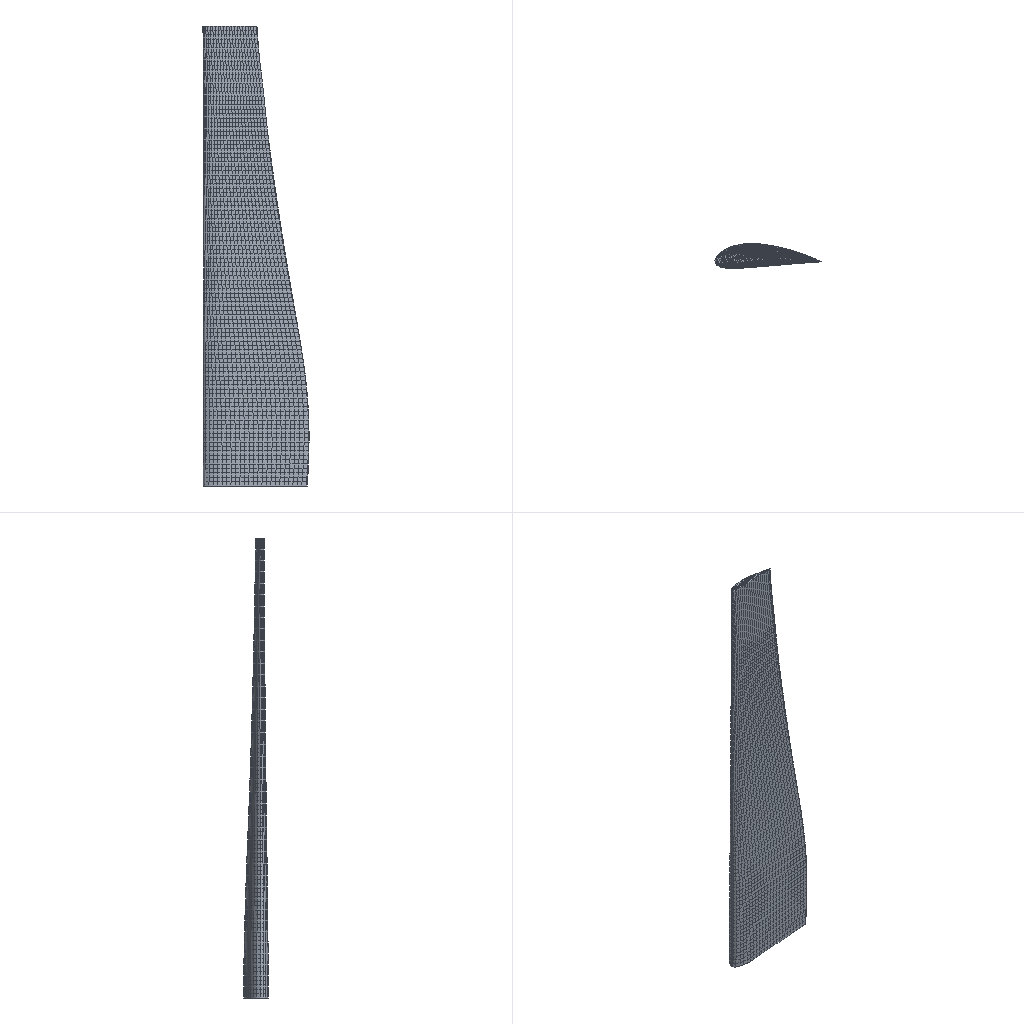Simulation study | abaqus
Set-up summary:
category,name,step,type,value,unit,region
solver,abaqus
solver,version,,,Abaqus/Standard 2020
units,not stated in the deck,,not stated
analysis,deck,,static,static
load_step,Step-1,Step-1,static,nlgeom=True
contact,interactions,,,general=0 pairs=0 ties=0
load_step,requested,,,1
mesh,nodes,,,20670
mesh,elements,,,17535
element_type,SC8R,,solid_shell,17535
load,load commands in deck,,count,1
bc,support commands in deck,,count,1
material,MATERIAL-1,,in results
check,setup vs results,,match,"per instance, exact: element labels, types and connectivity; labels of the nodes the elements use; coordinates of those nodes at SINGLE_PRECISION in 1 of 1 instance(s)"
Abaqus input file, long lists of numbers shortened:
*Heading
** Job name: Job-2 Model name: Model-1
** Generated by: Abaqus/CAE 2020
*Preprint, echo=NO, model=NO, history=NO, contact=NO
**
** PARTS
**
*Part, name="Blade 1"
*Node
      1,   238.218, 0.009342,         151.
      2,   235.201, -0.436,         151.
** (20668 more lines like these left out)
*Element, type=SC8R
    1,   323,    59,   321,   322,  8361,  2547,  8359,  8360
    2,   323,   322,   325,   324,  8361,  8360,  8363,  8362
** (17533 more lines like these left out)
*Nset, nset=Set-1, generate
     1,  20670,      1
*Elset, elset=Set-1, generate
     1,  17535,      1
*Orientation, name=Ori-2
          1.,           0.,           0.,           0.,           1.,           0.
3, 0.
** Region: (CompositeLayup-2-1: Generated From Layup)
*Elset, elset=CompositeLayup-2-1, generate
     1,  14805,      1
** Section: CompositeLayup-2-1
*Shell Section, elset=CompositeLayup-2-1, composite, orientation=Ori-2, stack direction=3, layup=CompositeLayup-2
1., 3, Material-1, 45., 层-1
*Orientation, name=Ori-3
          1.,           0.,           0.,           0.,           1.,           0.
3, 0.
** Region: (CompositeLayup-2-2: Generated From Layup)
*Elset, elset=CompositeLayup-2-2, generate
 14806,  17535,      1
** Section: CompositeLayup-2-2
*Shell Section, elset=CompositeLayup-2-2, composite, orientation=Ori-3, stack direction=3, layup=CompositeLayup-2
1., 3, Material-1, -45., 层-2
*End Part
**
**
** ASSEMBLY
**
*Assembly, name=Assembly
**
*Instance, name="Blade 1-1", part="Blade 1"
*End Instance
**
*Nset, nset=Set-1, instance="Blade 1-1"
    1,    2,    3,    4,    8,    9,   10,   11,   12,   13,   14,   15,   16,   17,   18,   19
   20,   21,   22,   23,   24,   25,   26,   27,   28,   29,   30,   31,   32,   33,   34,   35
** (11 more lines like these left out)
*Elset, elset=Set-1, instance="Blade 1-1"
     1,     2,     3,     4,     5,     6,     7,     8,     9,    10,    11,    12,    13,    14,    15,    16
    17,    18,    19,    20,    21,    22,    23,    24,    25,    26,    27,    28,    29,    30,    31,    32
** (9 more lines like these left out)
*Elset, elset=_Surf-1_S6, internal, instance="Blade 1-1"
     4,     5,     7,    10,    27,    31,    32,    34,    35,    36,    44,    45,    49,    62,    70,    72
    76,    85,    89,    90,   131,   145,   146,   148,   151,   168,   172,   173,   175,   176,   177,   185
** (136 more lines like these left out)
*Elset, elset=_Surf-1_S3, internal, instance="Blade 1-1"
     9,    24,    30,    33,    39,    40,    41,    67,   116,   123,   125,   130,   133,   150,   165,   171
   174,   180,   181,   182,   208,   257,   264,   266,   271,   274,   291,   306,   312,   315,   321,   322
** (84 more lines like these left out)
*Elset, elset=_Surf-1_S4, internal, instance="Blade 1-1"
    12,    66,    68,    75,    81,    86,    93,    96,    99,   111,   114,   117,   125,   153,   207,   209
   216,   222,   227,   234,   237,   240,   252,   255,   258,   266,   294,   348,   350,   357,   363,   368
** (84 more lines like these left out)
*Elset, elset=_Surf-1_S5, internal, instance="Blade 1-1"
    13,    60,   115,   122,   124,   128,   129,   154,   201,   256,   263,   265,   269,   270,   295,   342
   397,   404,   406,   410,   411,   436,   483,   538,   545,   547,   551,   552,   577,   624,   679,   686
** (44 more lines like these left out)
*Surface, type=ELEMENT, name=Surf-1
_Surf-1_S6, S6
_Surf-1_S3, S3
_Surf-1_S4, S4
_Surf-1_S5, S5
*End Assembly
*Amplitude, name=Amp-1
             0.,              0.,              1.,              1.
**
** MATERIALS
**
*Material, name=Material-1
*Density
1210.,
*Elastic, type=ENGINEERING CONSTANTS
 1.12e+11, 8.2e+09, 8.2e+09,     0.3,     0.3,     0.4, 4.5e+09, 4.5e+09
   3e+09,
** ----------------------------------------------------------------
**
** STEP: Step-1
**
*Step, name=Step-1, nlgeom=YES, inc=10000
*Static, stabilize=0.0002, allsdtol=0.05, continue=NO
0.001, 1., 1e-05, 1.
**
** BOUNDARY CONDITIONS
**
** Name: BC-1 Type: 对称/反对称/完全固定
*Boundary
Set-1, ENCASTRE
**
** LOADS
**
** Name: Load-1   Type: Pressure
*Dsload, amplitude=Amp-1
Surf-1, P, 1e+06
**
** OUTPUT REQUESTS
**
*Restart, write, frequency=0
**
** FIELD OUTPUT: F-Output-1
**
*Output, field
*Node Output
CF, RF, U, V
*Element Output, directions=YES
E, LE, MISES, PE, PEEQ, PEEQMAX, PEEQT, PEMAG, S, SE, VE, VEEQ
*Contact Output
CDISP, CSTRESS
**
** HISTORY OUTPUT: H-Output-1
**
*Output, history, variable=PRESELECT
*End Step
Results summary:
result,step,,completed,increments=27 time=1.0/1.0
result,analysis,,,static
result,last_loadstep,,,1
result,analysis steps,,count,1
result,primary field,,,U
result,reaction total,,FX,-1534843.641,model units
result,reaction total,,FY,-5415623.146,model units
result,reaction total,,FZ,7427711989.25,model units